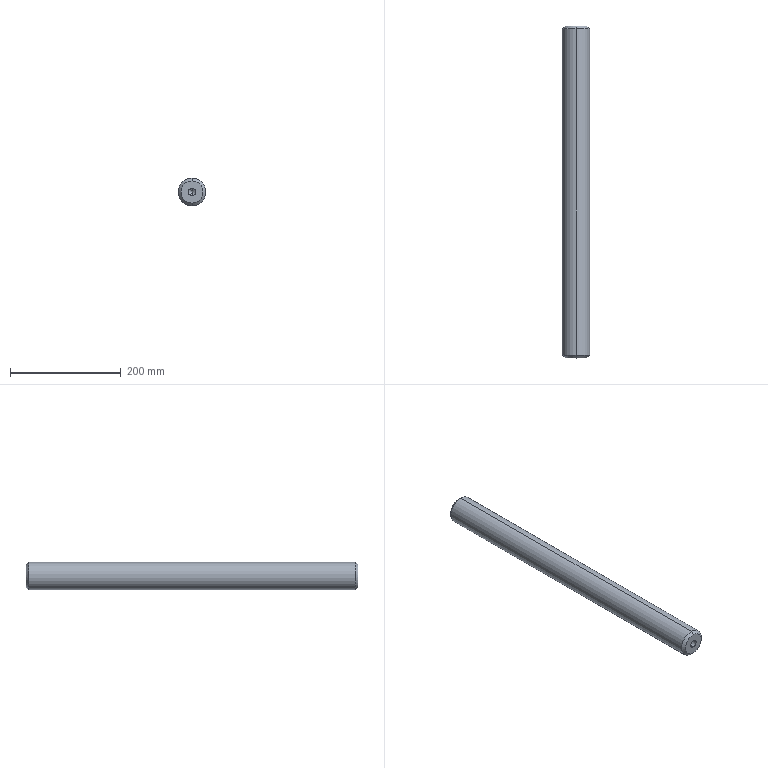Part | SolidWorks | features HoleWzd 2, Chamfer 1, Extrusion 1 | 1 solid | 16 faces | box 50 x 600 x 50 mm | volume 1162301 mm3 | cone 8 | cylinder 6 | plane 2 | commonest cylinder face diameters 14 x4 50 x2
STEP:
#1=CARTESIAN_POINT('',(0.,38.,7.));
#2=VERTEX_POINT('',#1);
#3=CARTESIAN_POINT('',(0.,38.,-7.));
#4=VERTEX_POINT('',#3);
#5=CARTESIAN_POINT('',(0.,38.,0.));
#6=DIRECTION('',(0.,-1.,0.));
#7=DIRECTION('',(0.,0.,-1.));
#8=AXIS2_PLACEMENT_3D('',#5,#6,#7);
#9=CIRCLE('',#8,7.);
#10=EDGE_CURVE('',#2,#4,#9,.T.);
#11=ORIENTED_EDGE('',*,*,#10,.F.);
#12=CARTESIAN_POINT('',(0.,0.,7.));
#13=VERTEX_POINT('',#12);
#14=CARTESIAN_POINT('',(0.,0.,7.));
#15=DIRECTION('',(0.,-1.,0.));
#16=VECTOR('',#15,1000.);
#17=LINE('',#14,#16);
#18=EDGE_CURVE('',#2,#13,#17,.T.);
#19=ORIENTED_EDGE('',*,*,#18,.T.);
#20=CARTESIAN_POINT('',(0.,0.,-7.));
#21=VERTEX_POINT('',#20);
#22=CARTESIAN_POINT('',(0.,0.,0.));
#23=DIRECTION('',(0.,-1.,0.));
#24=DIRECTION('',(0.,0.,-1.));
#25=AXIS2_PLACEMENT_3D('',#22,#23,#24);
#26=CIRCLE('',#25,7.);
#27=EDGE_CURVE('',#13,#21,#26,.T.);
#28=ORIENTED_EDGE('',*,*,#27,.T.);
#29=CARTESIAN_POINT('',(0.,0.,-7.));
#30=DIRECTION('',(0.,-1.,0.));
#31=VECTOR('',#30,1000.);
#32=LINE('',#29,#31);
#33=EDGE_CURVE('',#4,#21,#32,.T.);
#34=ORIENTED_EDGE('',*,*,#33,.F.);
#35=EDGE_LOOP('',(#11,#19,#28,#34));
#36=FACE_OUTER_BOUND('',#35,.T.);
#37=CARTESIAN_POINT('',(0.,0.,0.));
#38=DIRECTION('',(0.,-1.,0.));
#39=DIRECTION('',(0.,0.,-1.));
#40=AXIS2_PLACEMENT_3D('',#37,#38,#39);
#41=CYLINDRICAL_SURFACE('',#40,7.);
#42=ADVANCED_FACE('',(#36),#41,.F.);
#43=CARTESIAN_POINT('',(0.,42.206,0.));
#44=VERTEX_POINT('',#43);
#45=CARTESIAN_POINT('',(0.,38.,-7.));
#46=DIRECTION('',(0.,-0.515,-0.8572));
#47=VECTOR('',#46,1000.);
#48=LINE('',#45,#47);
#49=EDGE_CURVE('',#44,#4,#48,.T.);
#50=ORIENTED_EDGE('',*,*,#49,.F.);
#51=CARTESIAN_POINT('',(0.,38.,7.));
#52=DIRECTION('',(0.,-0.515,0.8572));
#53=VECTOR('',#52,1000.);
#54=LINE('',#51,#53);
#55=EDGE_CURVE('',#44,#2,#54,.T.);
#56=ORIENTED_EDGE('',*,*,#55,.T.);
#57=ORIENTED_EDGE('',*,*,#10,.T.);
#58=EDGE_LOOP('',(#50,#56,#57));
#59=FACE_OUTER_BOUND('',#58,.T.);
#60=CARTESIAN_POINT('',(0.,38.,0.));
#61=DIRECTION('',(0.,-1.,0.));
#62=DIRECTION('',(0.,0.,-1.));
#63=AXIS2_PLACEMENT_3D('',#60,#61,#62);
#64=CONICAL_SURFACE('',#63,7.,1.03);
#65=ADVANCED_FACE('',(#59),#64,.F.);
#66=CARTESIAN_POINT('',(0.,562.,-7.));
#67=VERTEX_POINT('',#66);
#68=CARTESIAN_POINT('',(0.,562.,7.));
#69=VERTEX_POINT('',#68);
#70=CARTESIAN_POINT('',(0.,562.,0.));
#71=DIRECTION('',(0.,1.,0.));
#72=DIRECTION('',(0.,0.,1.));
#73=AXIS2_PLACEMENT_3D('',#70,#71,#72);
#74=CIRCLE('',#73,7.);
#75=EDGE_CURVE('',#67,#69,#74,.T.);
#76=ORIENTED_EDGE('',*,*,#75,.F.);
#77=CARTESIAN_POINT('',(0.,600.,-7.));
#78=VERTEX_POINT('',#77);
#79=CARTESIAN_POINT('',(0.,600.,-7.));
#80=DIRECTION('',(0.,1.,0.));
#81=VECTOR('',#80,1000.);
#82=LINE('',#79,#81);
#83=EDGE_CURVE('',#67,#78,#82,.T.);
#84=ORIENTED_EDGE('',*,*,#83,.T.);
#85=CARTESIAN_POINT('',(0.,600.,7.));
#86=VERTEX_POINT('',#85);
#87=CARTESIAN_POINT('',(0.,600.,0.));
#88=DIRECTION('',(0.,1.,0.));
#89=DIRECTION('',(0.,0.,1.));
#90=AXIS2_PLACEMENT_3D('',#87,#88,#89);
#91=CIRCLE('',#90,7.);
#92=EDGE_CURVE('',#78,#86,#91,.T.);
#93=ORIENTED_EDGE('',*,*,#92,.T.);
#94=CARTESIAN_POINT('',(0.,600.,7.));
#95=DIRECTION('',(0.,1.,0.));
#96=VECTOR('',#95,1000.);
#97=LINE('',#94,#96);
#98=EDGE_CURVE('',#69,#86,#97,.T.);
#99=ORIENTED_EDGE('',*,*,#98,.F.);
#100=EDGE_LOOP('',(#76,#84,#93,#99));
#101=FACE_OUTER_BOUND('',#100,.T.);
#102=CARTESIAN_POINT('',(0.,600.,0.));
#103=DIRECTION('',(0.,1.,0.));
#104=DIRECTION('',(0.,0.,1.));
#105=AXIS2_PLACEMENT_3D('',#102,#103,#104);
#106=CYLINDRICAL_SURFACE('',#105,7.);
#107=ADVANCED_FACE('',(#101),#106,.F.);
#108=CARTESIAN_POINT('',(0.,557.794,0.));
#109=VERTEX_POINT('',#108);
#110=CARTESIAN_POINT('',(0.,562.,7.));
#111=DIRECTION('',(0.,0.515,0.8572));
#112=VECTOR('',#111,1000.);
#113=LINE('',#110,#112);
#114=EDGE_CURVE('',#109,#69,#113,.T.);
#115=ORIENTED_EDGE('',*,*,#114,.F.);
#116=CARTESIAN_POINT('',(0.,562.,-7.));
#117=DIRECTION('',(0.,0.515,-0.8572));
#118=VECTOR('',#117,1000.);
#119=LINE('',#116,#118);
#120=EDGE_CURVE('',#109,#67,#119,.T.);
#121=ORIENTED_EDGE('',*,*,#120,.T.);
#122=ORIENTED_EDGE('',*,*,#75,.T.);
#123=EDGE_LOOP('',(#115,#121,#122));
#124=FACE_OUTER_BOUND('',#123,.T.);
#125=CARTESIAN_POINT('',(0.,562.,0.));
#126=DIRECTION('',(0.,1.,0.));
#127=DIRECTION('',(0.,0.,1.));
#128=AXIS2_PLACEMENT_3D('',#125,#126,#127);
#129=CONICAL_SURFACE('',#128,7.,1.03);
#130=ADVANCED_FACE('',(#124),#129,.F.);
#131=CARTESIAN_POINT('',(0.,600.,20.));
#132=VERTEX_POINT('',#131);
#133=CARTESIAN_POINT('',(0.,600.,-20.));
#134=VERTEX_POINT('',#133);
#135=CARTESIAN_POINT('',(0.,600.,0.));
#136=DIRECTION('',(0.,1.,0.));
#137=DIRECTION('',(0.,0.,1.));
#138=AXIS2_PLACEMENT_3D('',#135,#136,#137);
#139=CIRCLE('',#138,20.);
#140=EDGE_CURVE('',#132,#134,#139,.T.);
#141=ORIENTED_EDGE('',*,*,#140,.F.);
#142=CARTESIAN_POINT('',(0.,595.,25.));
#143=VERTEX_POINT('',#142);
#144=CARTESIAN_POINT('',(0.,600.,20.));
#145=DIRECTION('',(0.,-0.7071,0.7071));
#146=VECTOR('',#145,1000.);
#147=LINE('',#144,#146);
#148=EDGE_CURVE('',#132,#143,#147,.T.);
#149=ORIENTED_EDGE('',*,*,#148,.T.);
#150=CARTESIAN_POINT('',(0.,595.,-25.));
#151=VERTEX_POINT('',#150);
#152=CARTESIAN_POINT('',(0.,595.,0.));
#153=DIRECTION('',(0.,-1.,0.));
#154=DIRECTION('',(0.,0.,1.));
#155=AXIS2_PLACEMENT_3D('',#152,#153,#154);
#156=CIRCLE('',#155,25.);
#157=EDGE_CURVE('',#151,#143,#156,.T.);
#158=ORIENTED_EDGE('',*,*,#157,.F.);
#159=CARTESIAN_POINT('',(0.,600.,-20.));
#160=DIRECTION('',(0.,-0.7071,-0.7071));
#161=VECTOR('',#160,1000.);
#162=LINE('',#159,#161);
#163=EDGE_CURVE('',#134,#151,#162,.T.);
#164=ORIENTED_EDGE('',*,*,#163,.F.);
#165=EDGE_LOOP('',(#141,#149,#158,#164));
#166=FACE_OUTER_BOUND('',#165,.T.);
#167=CARTESIAN_POINT('',(0.,600.,0.));
#168=DIRECTION('',(0.,-1.,0.));
#169=DIRECTION('',(0.,0.,-1.));
#170=AXIS2_PLACEMENT_3D('',#167,#168,#169);
#171=CONICAL_SURFACE('',#170,20.,0.7854);
#172=ADVANCED_FACE('',(#166),#171,.T.);
#173=CARTESIAN_POINT('',(0.,0.,-20.));
#174=VERTEX_POINT('',#173);
#175=CARTESIAN_POINT('',(0.,0.,20.));
#176=VERTEX_POINT('',#175);
#177=CARTESIAN_POINT('',(0.,0.,0.));
#178=DIRECTION('',(0.,-1.,0.));
#179=DIRECTION('',(0.,0.,1.));
#180=AXIS2_PLACEMENT_3D('',#177,#178,#179);
#181=CIRCLE('',#180,20.);
#182=EDGE_CURVE('',#174,#176,#181,.T.);
#183=ORIENTED_EDGE('',*,*,#182,.F.);
#184=CARTESIAN_POINT('',(0.,5.,-25.));
#185=VERTEX_POINT('',#184);
#186=CARTESIAN_POINT('',(0.,5.,-25.));
#187=DIRECTION('',(0.,0.7071,-0.7071));
#188=VECTOR('',#187,1000.);
#189=LINE('',#186,#188);
#190=EDGE_CURVE('',#174,#185,#189,.T.);
#191=ORIENTED_EDGE('',*,*,#190,.T.);
#192=CARTESIAN_POINT('',(0.,5.,25.));
#193=VERTEX_POINT('',#192);
#194=CARTESIAN_POINT('',(0.,5.,0.));
#195=DIRECTION('',(0.,1.,0.));
#196=DIRECTION('',(0.,0.,1.));
#197=AXIS2_PLACEMENT_3D('',#194,#195,#196);
#198=CIRCLE('',#197,25.);
#199=EDGE_CURVE('',#193,#185,#198,.T.);
#200=ORIENTED_EDGE('',*,*,#199,.F.);
#201=CARTESIAN_POINT('',(0.,5.,25.));
#202=DIRECTION('',(0.,0.7071,0.7071));
#203=VECTOR('',#202,1000.);
#204=LINE('',#201,#203);
#205=EDGE_CURVE('',#176,#193,#204,.T.);
#206=ORIENTED_EDGE('',*,*,#205,.F.);
#207=EDGE_LOOP('',(#183,#191,#200,#206));
#208=FACE_OUTER_BOUND('',#207,.T.);
#209=CARTESIAN_POINT('',(0.,5.,0.));
#210=DIRECTION('',(0.,1.,0.));
#211=DIRECTION('',(0.,0.,1.));
#212=AXIS2_PLACEMENT_3D('',#209,#210,#211);
#213=CONICAL_SURFACE('',#212,25.,0.7854);
#214=ADVANCED_FACE('',(#208),#213,.T.);
#215=ORIENTED_EDGE('',*,*,#157,.T.);
#216=CARTESIAN_POINT('',(0.,600.,25.));
#217=DIRECTION('',(0.,-1.,0.));
#218=VECTOR('',#217,1000.);
#219=LINE('',#216,#218);
#220=EDGE_CURVE('',#143,#193,#219,.T.);
#221=ORIENTED_EDGE('',*,*,#220,.T.);
#222=ORIENTED_EDGE('',*,*,#199,.T.);
#223=CARTESIAN_POINT('',(0.,600.,-25.));
#224=DIRECTION('',(0.,-1.,0.));
#225=VECTOR('',#224,1000.);
#226=LINE('',#223,#225);
#227=EDGE_CURVE('',#151,#185,#226,.T.);
#228=ORIENTED_EDGE('',*,*,#227,.F.);
#229=EDGE_LOOP('',(#215,#221,#222,#228));
#230=FACE_OUTER_BOUND('',#229,.T.);
#231=CARTESIAN_POINT('',(0.,600.,0.));
#232=DIRECTION('',(0.,-1.,0.));
#233=DIRECTION('',(0.,0.,-1.));
#234=AXIS2_PLACEMENT_3D('',#231,#232,#233);
#235=CYLINDRICAL_SURFACE('',#234,25.);
#236=ADVANCED_FACE('',(#230),#235,.T.);
#237=ORIENTED_EDGE('',*,*,#220,.F.);
#238=CARTESIAN_POINT('',(0.,595.,0.));
#239=DIRECTION('',(0.,-1.,0.));
#240=DIRECTION('',(0.,0.,1.));
#241=AXIS2_PLACEMENT_3D('',#238,#239,#240);
#242=CIRCLE('',#241,25.);
#243=EDGE_CURVE('',#143,#151,#242,.T.);
#244=ORIENTED_EDGE('',*,*,#243,.T.);
#245=ORIENTED_EDGE('',*,*,#227,.T.);
#246=CARTESIAN_POINT('',(0.,5.,0.));
#247=DIRECTION('',(0.,1.,0.));
#248=DIRECTION('',(0.,0.,1.));
#249=AXIS2_PLACEMENT_3D('',#246,#247,#248);
#250=CIRCLE('',#249,25.);
#251=EDGE_CURVE('',#185,#193,#250,.T.);
#252=ORIENTED_EDGE('',*,*,#251,.T.);
#253=EDGE_LOOP('',(#237,#244,#245,#252));
#254=FACE_OUTER_BOUND('',#253,.T.);
#255=CARTESIAN_POINT('',(0.,600.,0.));
#256=DIRECTION('',(0.,-1.,0.));
#257=DIRECTION('',(0.,0.,-1.));
#258=AXIS2_PLACEMENT_3D('',#255,#256,#257);
#259=CYLINDRICAL_SURFACE('',#258,25.);
#260=ADVANCED_FACE('',(#254),#259,.T.);
#261=CARTESIAN_POINT('',(0.,600.,0.));
#262=DIRECTION('',(0.,1.,0.));
#263=DIRECTION('',(0.,0.,1.));
#264=AXIS2_PLACEMENT_3D('',#261,#262,#263);
#265=CIRCLE('',#264,7.);
#266=EDGE_CURVE('',#86,#78,#265,.T.);
#267=ORIENTED_EDGE('',*,*,#266,.F.);
#268=ORIENTED_EDGE('',*,*,#92,.F.);
#269=EDGE_LOOP('',(#267,#268));
#270=FACE_BOUND('',#269,.T.);
#271=CARTESIAN_POINT('',(0.,600.,0.));
#272=DIRECTION('',(0.,1.,0.));
#273=DIRECTION('',(0.,0.,1.));
#274=AXIS2_PLACEMENT_3D('',#271,#272,#273);
#275=CIRCLE('',#274,20.);
#276=EDGE_CURVE('',#134,#132,#275,.T.);
#277=ORIENTED_EDGE('',*,*,#276,.T.);
#278=ORIENTED_EDGE('',*,*,#140,.T.);
#279=EDGE_LOOP('',(#277,#278));
#280=FACE_OUTER_BOUND('',#279,.T.);
#281=CARTESIAN_POINT('',(0.,600.,0.));
#282=DIRECTION('',(0.,1.,0.));
#283=DIRECTION('',(0.,0.,1.));
#284=AXIS2_PLACEMENT_3D('',#281,#282,#283);
#285=PLANE('',#284);
#286=ADVANCED_FACE('',(#270,#280),#285,.T.);
#287=CARTESIAN_POINT('',(0.,0.,0.));
#288=DIRECTION('',(0.,-1.,0.));
#289=DIRECTION('',(0.,0.,-1.));
#290=AXIS2_PLACEMENT_3D('',#287,#288,#289);
#291=CIRCLE('',#290,7.);
#292=EDGE_CURVE('',#21,#13,#291,.T.);
#293=ORIENTED_EDGE('',*,*,#292,.F.);
#294=ORIENTED_EDGE('',*,*,#27,.F.);
#295=EDGE_LOOP('',(#293,#294));
#296=FACE_BOUND('',#295,.T.);
#297=CARTESIAN_POINT('',(0.,0.,0.));
#298=DIRECTION('',(0.,-1.,0.));
#299=DIRECTION('',(0.,0.,1.));
#300=AXIS2_PLACEMENT_3D('',#297,#298,#299);
#301=CIRCLE('',#300,20.);
#302=EDGE_CURVE('',#176,#174,#301,.T.);
#303=ORIENTED_EDGE('',*,*,#302,.T.);
#304=ORIENTED_EDGE('',*,*,#182,.T.);
#305=EDGE_LOOP('',(#303,#304));
#306=FACE_OUTER_BOUND('',#305,.T.);
#307=CARTESIAN_POINT('',(0.,0.,0.));
#308=DIRECTION('',(0.,1.,0.));
#309=DIRECTION('',(0.,0.,1.));
#310=AXIS2_PLACEMENT_3D('',#307,#308,#309);
#311=PLANE('',#310);
#312=ADVANCED_FACE('',(#296,#306),#311,.F.);
#313=ORIENTED_EDGE('',*,*,#190,.F.);
#314=ORIENTED_EDGE('',*,*,#302,.F.);
#315=ORIENTED_EDGE('',*,*,#205,.T.);
#316=ORIENTED_EDGE('',*,*,#251,.F.);
#317=EDGE_LOOP('',(#313,#314,#315,#316));
#318=FACE_OUTER_BOUND('',#317,.T.);
#319=CARTESIAN_POINT('',(0.,5.,0.));
#320=DIRECTION('',(0.,1.,0.));
#321=DIRECTION('',(0.,0.,1.));
#322=AXIS2_PLACEMENT_3D('',#319,#320,#321);
#323=CONICAL_SURFACE('',#322,25.,0.7854);
#324=ADVANCED_FACE('',(#318),#323,.T.);
#325=ORIENTED_EDGE('',*,*,#148,.F.);
#326=ORIENTED_EDGE('',*,*,#276,.F.);
#327=ORIENTED_EDGE('',*,*,#163,.T.);
#328=ORIENTED_EDGE('',*,*,#243,.F.);
#329=EDGE_LOOP('',(#325,#326,#327,#328));
#330=FACE_OUTER_BOUND('',#329,.T.);
#331=CARTESIAN_POINT('',(0.,600.,0.));
#332=DIRECTION('',(0.,-1.,0.));
#333=DIRECTION('',(0.,0.,-1.));
#334=AXIS2_PLACEMENT_3D('',#331,#332,#333);
#335=CONICAL_SURFACE('',#334,20.,0.7854);
#336=ADVANCED_FACE('',(#330),#335,.T.);
#337=ORIENTED_EDGE('',*,*,#120,.F.);
#338=ORIENTED_EDGE('',*,*,#114,.T.);
#339=CARTESIAN_POINT('',(0.,562.,0.));
#340=DIRECTION('',(0.,1.,0.));
#341=DIRECTION('',(0.,0.,1.));
#342=AXIS2_PLACEMENT_3D('',#339,#340,#341);
#343=CIRCLE('',#342,7.);
#344=EDGE_CURVE('',#69,#67,#343,.T.);
#345=ORIENTED_EDGE('',*,*,#344,.T.);
#346=EDGE_LOOP('',(#337,#338,#345));
#347=FACE_OUTER_BOUND('',#346,.T.);
#348=CARTESIAN_POINT('',(0.,562.,0.));
#349=DIRECTION('',(0.,1.,0.));
#350=DIRECTION('',(0.,0.,1.));
#351=AXIS2_PLACEMENT_3D('',#348,#349,#350);
#352=CONICAL_SURFACE('',#351,7.,1.03);
#353=ADVANCED_FACE('',(#347),#352,.F.);
#354=ORIENTED_EDGE('',*,*,#83,.F.);
#355=ORIENTED_EDGE('',*,*,#344,.F.);
#356=ORIENTED_EDGE('',*,*,#98,.T.);
#357=ORIENTED_EDGE('',*,*,#266,.T.);
#358=EDGE_LOOP('',(#354,#355,#356,#357));
#359=FACE_OUTER_BOUND('',#358,.T.);
#360=CARTESIAN_POINT('',(0.,600.,0.));
#361=DIRECTION('',(0.,1.,0.));
#362=DIRECTION('',(0.,0.,1.));
#363=AXIS2_PLACEMENT_3D('',#360,#361,#362);
#364=CYLINDRICAL_SURFACE('',#363,7.);
#365=ADVANCED_FACE('',(#359),#364,.F.);
#366=ORIENTED_EDGE('',*,*,#55,.F.);
#367=ORIENTED_EDGE('',*,*,#49,.T.);
#368=CARTESIAN_POINT('',(0.,38.,0.));
#369=DIRECTION('',(0.,-1.,0.));
#370=DIRECTION('',(0.,0.,-1.));
#371=AXIS2_PLACEMENT_3D('',#368,#369,#370);
#372=CIRCLE('',#371,7.);
#373=EDGE_CURVE('',#4,#2,#372,.T.);
#374=ORIENTED_EDGE('',*,*,#373,.T.);
#375=EDGE_LOOP('',(#366,#367,#374));
#376=FACE_OUTER_BOUND('',#375,.T.);
#377=CARTESIAN_POINT('',(0.,38.,0.));
#378=DIRECTION('',(0.,-1.,0.));
#379=DIRECTION('',(0.,0.,-1.));
#380=AXIS2_PLACEMENT_3D('',#377,#378,#379);
#381=CONICAL_SURFACE('',#380,7.,1.03);
#382=ADVANCED_FACE('',(#376),#381,.F.);
#383=ORIENTED_EDGE('',*,*,#18,.F.);
#384=ORIENTED_EDGE('',*,*,#373,.F.);
#385=ORIENTED_EDGE('',*,*,#33,.T.);
#386=ORIENTED_EDGE('',*,*,#292,.T.);
#387=EDGE_LOOP('',(#383,#384,#385,#386));
#388=FACE_OUTER_BOUND('',#387,.T.);
#389=CARTESIAN_POINT('',(0.,0.,0.));
#390=DIRECTION('',(0.,-1.,0.));
#391=DIRECTION('',(0.,0.,-1.));
#392=AXIS2_PLACEMENT_3D('',#389,#390,#391);
#393=CYLINDRICAL_SURFACE('',#392,7.);
#394=ADVANCED_FACE('',(#388),#393,.F.);
#395=CLOSED_SHELL('',(#42,#65,#107,#130,#172,#214,#236,#260,#286,#312,#324,#336,#353,#365,#382,#394));
#396=MANIFOLD_SOLID_BREP('',#395);
#397=CARTESIAN_POINT('',(0.,0.,0.));
#398=DIRECTION('',(0.,0.,1.));
#399=DIRECTION('',(1.,0.,0.));
#400=AXIS2_PLACEMENT_3D('',#397,#398,#399);
#401=(LENGTH_UNIT()NAMED_UNIT(*)SI_UNIT(.MILLI.,.METRE.));
#402=UNCERTAINTY_MEASURE_WITH_UNIT(LENGTH_MEASURE(0.00001),#401,'','');
#403=(NAMED_UNIT(*)PLANE_ANGLE_UNIT()SI_UNIT($,.RADIAN.));
#404=(NAMED_UNIT(*)SI_UNIT($,.STERADIAN.)SOLID_ANGLE_UNIT());
#405=(GEOMETRIC_REPRESENTATION_CONTEXT(3)GLOBAL_UNCERTAINTY_ASSIGNED_CONTEXT((#402))GLOBAL_UNIT_ASSIGNED_CONTEXT((#401,#403,#404))REPRESENTATION_CONTEXT('',''));
#406=ADVANCED_BREP_SHAPE_REPRESENTATION('',(#396,#400),#405);